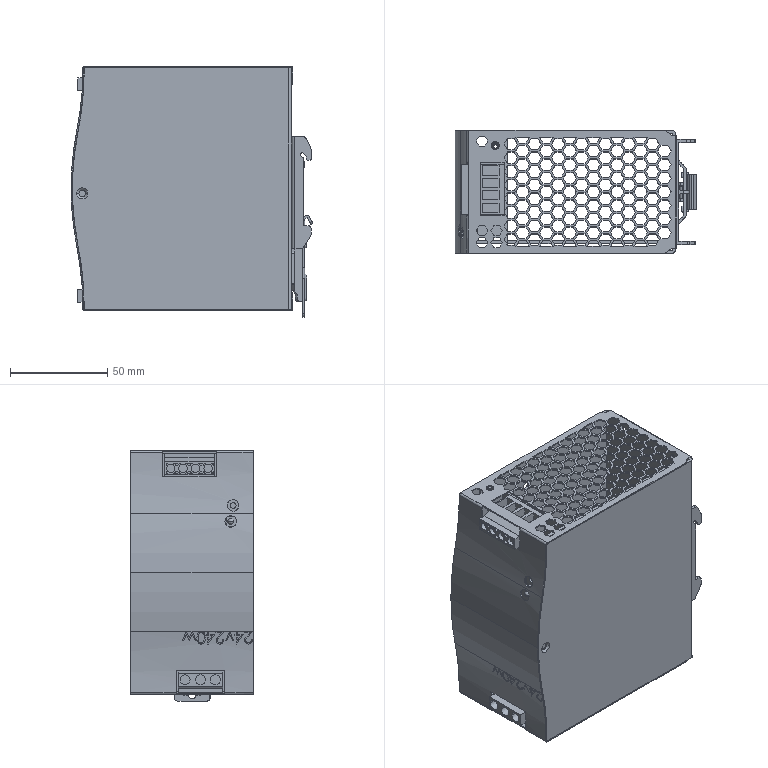Part | STEP file | rail switch-mode power supply NDR-240-24 | 12 solids | 2299 faces | box 124.256 x 63 x 128.712 mm | volume 109932 mm3 | plane 1928 | cylinder 278 | cone 42 | spline 41 | torus 8 | other 2 | commonest cylinder face diameters 2 x41 3.4 x28 4 x24 1 x23 0.2 x22 6 x20